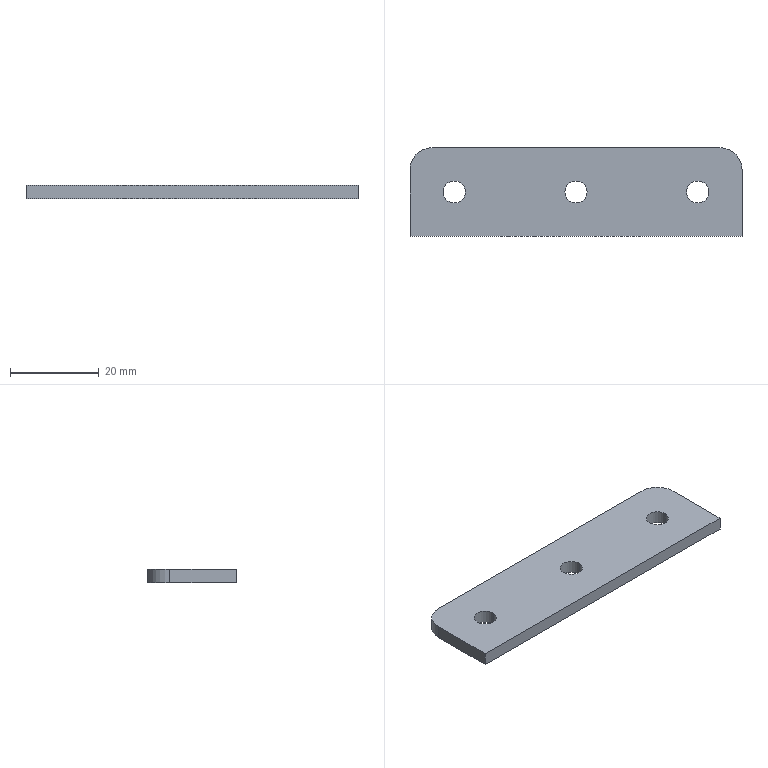Part | SolidWorks | features Extrusion 1, Fillet 1 | 1 solid | 14 faces | box 75 x 20 x 3 mm | volume 4291 mm3 | cylinder 8 | plane 6 | commonest cylinder face diameters 5 x6 10 x2
STEP:
#1=CARTESIAN_POINT('',(62.5,-10.,3.));
#2=VERTEX_POINT('',#1);
#3=CARTESIAN_POINT('',(67.5,-10.,3.));
#4=VERTEX_POINT('',#3);
#5=CARTESIAN_POINT('',(65.,-10.,3.));
#6=DIRECTION('',(0.,0.,1.));
#7=DIRECTION('',(1.,0.,0.));
#8=AXIS2_PLACEMENT_3D('',#5,#6,#7);
#9=CIRCLE('',#8,2.5);
#10=EDGE_CURVE('',#2,#4,#9,.T.);
#11=ORIENTED_EDGE('',*,*,#10,.T.);
#12=CARTESIAN_POINT('',(67.5,-10.,0.));
#13=VERTEX_POINT('',#12);
#14=CARTESIAN_POINT('',(67.5,-10.,3.));
#15=DIRECTION('',(0.,0.,-1.));
#16=VECTOR('',#15,1000.);
#17=LINE('',#14,#16);
#18=EDGE_CURVE('',#4,#13,#17,.T.);
#19=ORIENTED_EDGE('',*,*,#18,.T.);
#20=CARTESIAN_POINT('',(62.5,-10.,0.));
#21=VERTEX_POINT('',#20);
#22=CARTESIAN_POINT('',(65.,-10.,0.));
#23=DIRECTION('',(0.,0.,1.));
#24=DIRECTION('',(1.,0.,0.));
#25=AXIS2_PLACEMENT_3D('',#22,#23,#24);
#26=CIRCLE('',#25,2.5);
#27=EDGE_CURVE('',#21,#13,#26,.T.);
#28=ORIENTED_EDGE('',*,*,#27,.F.);
#29=CARTESIAN_POINT('',(62.5,-10.,3.));
#30=DIRECTION('',(0.,0.,-1.));
#31=VECTOR('',#30,1000.);
#32=LINE('',#29,#31);
#33=EDGE_CURVE('',#2,#21,#32,.T.);
#34=ORIENTED_EDGE('',*,*,#33,.F.);
#35=EDGE_LOOP('',(#11,#19,#28,#34));
#36=FACE_OUTER_BOUND('',#35,.T.);
#37=CARTESIAN_POINT('',(65.,-10.,3.));
#38=DIRECTION('',(0.,0.,-1.));
#39=DIRECTION('',(-1.,0.,0.));
#40=AXIS2_PLACEMENT_3D('',#37,#38,#39);
#41=CYLINDRICAL_SURFACE('',#40,2.5);
#42=ADVANCED_FACE('',(#36),#41,.F.);
#43=CARTESIAN_POINT('',(35.,-10.,3.));
#44=VERTEX_POINT('',#43);
#45=CARTESIAN_POINT('',(40.,-10.,3.));
#46=VERTEX_POINT('',#45);
#47=CARTESIAN_POINT('',(37.5,-10.,3.));
#48=DIRECTION('',(0.,0.,1.));
#49=DIRECTION('',(1.,0.,0.));
#50=AXIS2_PLACEMENT_3D('',#47,#48,#49);
#51=CIRCLE('',#50,2.5);
#52=EDGE_CURVE('',#44,#46,#51,.T.);
#53=ORIENTED_EDGE('',*,*,#52,.T.);
#54=CARTESIAN_POINT('',(40.,-10.,0.));
#55=VERTEX_POINT('',#54);
#56=CARTESIAN_POINT('',(40.,-10.,3.));
#57=DIRECTION('',(0.,0.,-1.));
#58=VECTOR('',#57,1000.);
#59=LINE('',#56,#58);
#60=EDGE_CURVE('',#46,#55,#59,.T.);
#61=ORIENTED_EDGE('',*,*,#60,.T.);
#62=CARTESIAN_POINT('',(35.,-10.,0.));
#63=VERTEX_POINT('',#62);
#64=CARTESIAN_POINT('',(37.5,-10.,0.));
#65=DIRECTION('',(0.,0.,1.));
#66=DIRECTION('',(1.,0.,0.));
#67=AXIS2_PLACEMENT_3D('',#64,#65,#66);
#68=CIRCLE('',#67,2.5);
#69=EDGE_CURVE('',#63,#55,#68,.T.);
#70=ORIENTED_EDGE('',*,*,#69,.F.);
#71=CARTESIAN_POINT('',(35.,-10.,3.));
#72=DIRECTION('',(0.,0.,-1.));
#73=VECTOR('',#72,1000.);
#74=LINE('',#71,#73);
#75=EDGE_CURVE('',#44,#63,#74,.T.);
#76=ORIENTED_EDGE('',*,*,#75,.F.);
#77=EDGE_LOOP('',(#53,#61,#70,#76));
#78=FACE_OUTER_BOUND('',#77,.T.);
#79=CARTESIAN_POINT('',(37.5,-10.,3.));
#80=DIRECTION('',(0.,0.,-1.));
#81=DIRECTION('',(-1.,0.,0.));
#82=AXIS2_PLACEMENT_3D('',#79,#80,#81);
#83=CYLINDRICAL_SURFACE('',#82,2.5);
#84=ADVANCED_FACE('',(#78),#83,.F.);
#85=CARTESIAN_POINT('',(7.5,-10.,3.));
#86=VERTEX_POINT('',#85);
#87=CARTESIAN_POINT('',(12.5,-10.,3.));
#88=VERTEX_POINT('',#87);
#89=CARTESIAN_POINT('',(10.,-10.,3.));
#90=DIRECTION('',(0.,0.,1.));
#91=DIRECTION('',(1.,0.,0.));
#92=AXIS2_PLACEMENT_3D('',#89,#90,#91);
#93=CIRCLE('',#92,2.5);
#94=EDGE_CURVE('',#86,#88,#93,.T.);
#95=ORIENTED_EDGE('',*,*,#94,.T.);
#96=CARTESIAN_POINT('',(12.5,-10.,0.));
#97=VERTEX_POINT('',#96);
#98=CARTESIAN_POINT('',(12.5,-10.,3.));
#99=DIRECTION('',(0.,0.,-1.));
#100=VECTOR('',#99,1000.);
#101=LINE('',#98,#100);
#102=EDGE_CURVE('',#88,#97,#101,.T.);
#103=ORIENTED_EDGE('',*,*,#102,.T.);
#104=CARTESIAN_POINT('',(7.5,-10.,0.));
#105=VERTEX_POINT('',#104);
#106=CARTESIAN_POINT('',(10.,-10.,0.));
#107=DIRECTION('',(0.,0.,1.));
#108=DIRECTION('',(1.,0.,0.));
#109=AXIS2_PLACEMENT_3D('',#106,#107,#108);
#110=CIRCLE('',#109,2.5);
#111=EDGE_CURVE('',#105,#97,#110,.T.);
#112=ORIENTED_EDGE('',*,*,#111,.F.);
#113=CARTESIAN_POINT('',(7.5,-10.,3.));
#114=DIRECTION('',(0.,0.,-1.));
#115=VECTOR('',#114,1000.);
#116=LINE('',#113,#115);
#117=EDGE_CURVE('',#86,#105,#116,.T.);
#118=ORIENTED_EDGE('',*,*,#117,.F.);
#119=EDGE_LOOP('',(#95,#103,#112,#118));
#120=FACE_OUTER_BOUND('',#119,.T.);
#121=CARTESIAN_POINT('',(10.,-10.,3.));
#122=DIRECTION('',(0.,0.,-1.));
#123=DIRECTION('',(-1.,0.,0.));
#124=AXIS2_PLACEMENT_3D('',#121,#122,#123);
#125=CYLINDRICAL_SURFACE('',#124,2.5);
#126=ADVANCED_FACE('',(#120),#125,.F.);
#127=ORIENTED_EDGE('',*,*,#52,.F.);
#128=CARTESIAN_POINT('',(37.5,-10.,3.));
#129=DIRECTION('',(0.,0.,1.));
#130=DIRECTION('',(1.,0.,0.));
#131=AXIS2_PLACEMENT_3D('',#128,#129,#130);
#132=CIRCLE('',#131,2.5);
#133=EDGE_CURVE('',#46,#44,#132,.T.);
#134=ORIENTED_EDGE('',*,*,#133,.F.);
#135=EDGE_LOOP('',(#127,#134));
#136=FACE_BOUND('',#135,.T.);
#137=CARTESIAN_POINT('',(75.,-20.,3.));
#138=VERTEX_POINT('',#137);
#139=CARTESIAN_POINT('',(75.,-5.,3.));
#140=VERTEX_POINT('',#139);
#141=CARTESIAN_POINT('',(75.,0.,3.));
#142=DIRECTION('',(0.,1.,0.));
#143=VECTOR('',#142,1000.);
#144=LINE('',#141,#143);
#145=EDGE_CURVE('',#138,#140,#144,.T.);
#146=ORIENTED_EDGE('',*,*,#145,.T.);
#147=CARTESIAN_POINT('',(70.,0.,3.));
#148=VERTEX_POINT('',#147);
#149=CARTESIAN_POINT('',(70.,-5.,3.));
#150=DIRECTION('',(0.,0.,1.));
#151=DIRECTION('',(1.,0.,0.));
#152=AXIS2_PLACEMENT_3D('',#149,#150,#151);
#153=CIRCLE('',#152,5.);
#154=EDGE_CURVE('',#140,#148,#153,.T.);
#155=ORIENTED_EDGE('',*,*,#154,.T.);
#156=CARTESIAN_POINT('',(5.,0.,3.));
#157=VERTEX_POINT('',#156);
#158=CARTESIAN_POINT('',(0.,0.,3.));
#159=DIRECTION('',(-1.,0.,0.));
#160=VECTOR('',#159,1000.);
#161=LINE('',#158,#160);
#162=EDGE_CURVE('',#148,#157,#161,.T.);
#163=ORIENTED_EDGE('',*,*,#162,.T.);
#164=CARTESIAN_POINT('',(0.,-5.,3.));
#165=VERTEX_POINT('',#164);
#166=CARTESIAN_POINT('',(5.,-5.,3.));
#167=DIRECTION('',(0.,0.,1.));
#168=DIRECTION('',(1.,0.,0.));
#169=AXIS2_PLACEMENT_3D('',#166,#167,#168);
#170=CIRCLE('',#169,5.);
#171=EDGE_CURVE('',#157,#165,#170,.T.);
#172=ORIENTED_EDGE('',*,*,#171,.T.);
#173=CARTESIAN_POINT('',(0.,-20.,3.));
#174=VERTEX_POINT('',#173);
#175=CARTESIAN_POINT('',(0.,0.,3.));
#176=DIRECTION('',(0.,-1.,0.));
#177=VECTOR('',#176,1000.);
#178=LINE('',#175,#177);
#179=EDGE_CURVE('',#165,#174,#178,.T.);
#180=ORIENTED_EDGE('',*,*,#179,.T.);
#181=CARTESIAN_POINT('',(0.,-20.,3.));
#182=DIRECTION('',(1.,0.,0.));
#183=VECTOR('',#182,1000.);
#184=LINE('',#181,#183);
#185=EDGE_CURVE('',#174,#138,#184,.T.);
#186=ORIENTED_EDGE('',*,*,#185,.T.);
#187=EDGE_LOOP('',(#146,#155,#163,#172,#180,#186));
#188=FACE_OUTER_BOUND('',#187,.T.);
#189=ORIENTED_EDGE('',*,*,#94,.F.);
#190=CARTESIAN_POINT('',(10.,-10.,3.));
#191=DIRECTION('',(0.,0.,1.));
#192=DIRECTION('',(1.,0.,0.));
#193=AXIS2_PLACEMENT_3D('',#190,#191,#192);
#194=CIRCLE('',#193,2.5);
#195=EDGE_CURVE('',#88,#86,#194,.T.);
#196=ORIENTED_EDGE('',*,*,#195,.F.);
#197=EDGE_LOOP('',(#189,#196));
#198=FACE_BOUND('',#197,.T.);
#199=ORIENTED_EDGE('',*,*,#10,.F.);
#200=CARTESIAN_POINT('',(65.,-10.,3.));
#201=DIRECTION('',(0.,0.,1.));
#202=DIRECTION('',(1.,0.,0.));
#203=AXIS2_PLACEMENT_3D('',#200,#201,#202);
#204=CIRCLE('',#203,2.5);
#205=EDGE_CURVE('',#4,#2,#204,.T.);
#206=ORIENTED_EDGE('',*,*,#205,.F.);
#207=EDGE_LOOP('',(#199,#206));
#208=FACE_BOUND('',#207,.T.);
#209=CARTESIAN_POINT('',(0.,0.,3.));
#210=DIRECTION('',(0.,0.,1.));
#211=DIRECTION('',(1.,0.,0.));
#212=AXIS2_PLACEMENT_3D('',#209,#210,#211);
#213=PLANE('',#212);
#214=ADVANCED_FACE('',(#136,#188,#198,#208),#213,.T.);
#215=CARTESIAN_POINT('',(70.,0.,0.));
#216=VERTEX_POINT('',#215);
#217=CARTESIAN_POINT('',(5.,0.,0.));
#218=VERTEX_POINT('',#217);
#219=CARTESIAN_POINT('',(0.,0.,0.));
#220=DIRECTION('',(-1.,0.,0.));
#221=VECTOR('',#220,1000.);
#222=LINE('',#219,#221);
#223=EDGE_CURVE('',#216,#218,#222,.T.);
#224=ORIENTED_EDGE('',*,*,#223,.F.);
#225=CARTESIAN_POINT('',(75.,-5.,0.));
#226=VERTEX_POINT('',#225);
#227=CARTESIAN_POINT('',(70.,-5.,0.));
#228=DIRECTION('',(0.,0.,-1.));
#229=DIRECTION('',(1.,0.,0.));
#230=AXIS2_PLACEMENT_3D('',#227,#228,#229);
#231=CIRCLE('',#230,5.);
#232=EDGE_CURVE('',#216,#226,#231,.T.);
#233=ORIENTED_EDGE('',*,*,#232,.T.);
#234=CARTESIAN_POINT('',(75.,-20.,0.));
#235=VERTEX_POINT('',#234);
#236=CARTESIAN_POINT('',(75.,0.,0.));
#237=DIRECTION('',(0.,1.,0.));
#238=VECTOR('',#237,1000.);
#239=LINE('',#236,#238);
#240=EDGE_CURVE('',#235,#226,#239,.T.);
#241=ORIENTED_EDGE('',*,*,#240,.F.);
#242=CARTESIAN_POINT('',(0.,-20.,0.));
#243=VERTEX_POINT('',#242);
#244=CARTESIAN_POINT('',(0.,-20.,0.));
#245=DIRECTION('',(1.,0.,0.));
#246=VECTOR('',#245,1000.);
#247=LINE('',#244,#246);
#248=EDGE_CURVE('',#243,#235,#247,.T.);
#249=ORIENTED_EDGE('',*,*,#248,.F.);
#250=CARTESIAN_POINT('',(0.,-5.,0.));
#251=VERTEX_POINT('',#250);
#252=CARTESIAN_POINT('',(0.,0.,0.));
#253=DIRECTION('',(0.,-1.,0.));
#254=VECTOR('',#253,1000.);
#255=LINE('',#252,#254);
#256=EDGE_CURVE('',#251,#243,#255,.T.);
#257=ORIENTED_EDGE('',*,*,#256,.F.);
#258=CARTESIAN_POINT('',(5.,-5.,0.));
#259=DIRECTION('',(0.,0.,-1.));
#260=DIRECTION('',(1.,0.,0.));
#261=AXIS2_PLACEMENT_3D('',#258,#259,#260);
#262=CIRCLE('',#261,5.);
#263=EDGE_CURVE('',#251,#218,#262,.T.);
#264=ORIENTED_EDGE('',*,*,#263,.T.);
#265=EDGE_LOOP('',(#224,#233,#241,#249,#257,#264));
#266=FACE_OUTER_BOUND('',#265,.T.);
#267=ORIENTED_EDGE('',*,*,#111,.T.);
#268=CARTESIAN_POINT('',(10.,-10.,0.));
#269=DIRECTION('',(0.,0.,1.));
#270=DIRECTION('',(1.,0.,0.));
#271=AXIS2_PLACEMENT_3D('',#268,#269,#270);
#272=CIRCLE('',#271,2.5);
#273=EDGE_CURVE('',#97,#105,#272,.T.);
#274=ORIENTED_EDGE('',*,*,#273,.T.);
#275=EDGE_LOOP('',(#267,#274));
#276=FACE_BOUND('',#275,.T.);
#277=ORIENTED_EDGE('',*,*,#69,.T.);
#278=CARTESIAN_POINT('',(37.5,-10.,0.));
#279=DIRECTION('',(0.,0.,1.));
#280=DIRECTION('',(1.,0.,0.));
#281=AXIS2_PLACEMENT_3D('',#278,#279,#280);
#282=CIRCLE('',#281,2.5);
#283=EDGE_CURVE('',#55,#63,#282,.T.);
#284=ORIENTED_EDGE('',*,*,#283,.T.);
#285=EDGE_LOOP('',(#277,#284));
#286=FACE_BOUND('',#285,.T.);
#287=ORIENTED_EDGE('',*,*,#27,.T.);
#288=CARTESIAN_POINT('',(65.,-10.,0.));
#289=DIRECTION('',(0.,0.,1.));
#290=DIRECTION('',(1.,0.,0.));
#291=AXIS2_PLACEMENT_3D('',#288,#289,#290);
#292=CIRCLE('',#291,2.5);
#293=EDGE_CURVE('',#13,#21,#292,.T.);
#294=ORIENTED_EDGE('',*,*,#293,.T.);
#295=EDGE_LOOP('',(#287,#294));
#296=FACE_BOUND('',#295,.T.);
#297=CARTESIAN_POINT('',(0.,0.,0.));
#298=DIRECTION('',(0.,0.,1.));
#299=DIRECTION('',(1.,0.,0.));
#300=AXIS2_PLACEMENT_3D('',#297,#298,#299);
#301=PLANE('',#300);
#302=ADVANCED_FACE('',(#266,#276,#286,#296),#301,.F.);
#303=ORIENTED_EDGE('',*,*,#179,.F.);
#304=CARTESIAN_POINT('',(0.,-5.,3.));
#305=DIRECTION('',(0.,0.,-1.));
#306=VECTOR('',#305,1000.);
#307=LINE('',#304,#306);
#308=EDGE_CURVE('',#165,#251,#307,.T.);
#309=ORIENTED_EDGE('',*,*,#308,.T.);
#310=ORIENTED_EDGE('',*,*,#256,.T.);
#311=CARTESIAN_POINT('',(0.,-20.,3.));
#312=DIRECTION('',(0.,0.,-1.));
#313=VECTOR('',#312,1000.);
#314=LINE('',#311,#313);
#315=EDGE_CURVE('',#174,#243,#314,.T.);
#316=ORIENTED_EDGE('',*,*,#315,.F.);
#317=EDGE_LOOP('',(#303,#309,#310,#316));
#318=FACE_OUTER_BOUND('',#317,.T.);
#319=CARTESIAN_POINT('',(0.,0.,3.));
#320=DIRECTION('',(1.,0.,0.));
#321=DIRECTION('',(0.,1.,0.));
#322=AXIS2_PLACEMENT_3D('',#319,#320,#321);
#323=PLANE('',#322);
#324=ADVANCED_FACE('',(#318),#323,.F.);
#325=ORIENTED_EDGE('',*,*,#248,.T.);
#326=CARTESIAN_POINT('',(75.,-20.,3.));
#327=DIRECTION('',(0.,0.,-1.));
#328=VECTOR('',#327,1000.);
#329=LINE('',#326,#328);
#330=EDGE_CURVE('',#138,#235,#329,.T.);
#331=ORIENTED_EDGE('',*,*,#330,.F.);
#332=ORIENTED_EDGE('',*,*,#185,.F.);
#333=ORIENTED_EDGE('',*,*,#315,.T.);
#334=EDGE_LOOP('',(#325,#331,#332,#333));
#335=FACE_OUTER_BOUND('',#334,.T.);
#336=CARTESIAN_POINT('',(0.,-20.,3.));
#337=DIRECTION('',(0.,1.,0.));
#338=DIRECTION('',(0.,0.,1.));
#339=AXIS2_PLACEMENT_3D('',#336,#337,#338);
#340=PLANE('',#339);
#341=ADVANCED_FACE('',(#335),#340,.F.);
#342=ORIENTED_EDGE('',*,*,#240,.T.);
#343=CARTESIAN_POINT('',(75.,-5.,3.));
#344=DIRECTION('',(0.,0.,1.));
#345=VECTOR('',#344,1000.);
#346=LINE('',#343,#345);
#347=EDGE_CURVE('',#226,#140,#346,.T.);
#348=ORIENTED_EDGE('',*,*,#347,.T.);
#349=ORIENTED_EDGE('',*,*,#145,.F.);
#350=ORIENTED_EDGE('',*,*,#330,.T.);
#351=EDGE_LOOP('',(#342,#348,#349,#350));
#352=FACE_OUTER_BOUND('',#351,.T.);
#353=CARTESIAN_POINT('',(75.,0.,3.));
#354=DIRECTION('',(-1.,0.,0.));
#355=DIRECTION('',(0.,0.,1.));
#356=AXIS2_PLACEMENT_3D('',#353,#354,#355);
#357=PLANE('',#356);
#358=ADVANCED_FACE('',(#352),#357,.F.);
#359=ORIENTED_EDGE('',*,*,#162,.F.);
#360=CARTESIAN_POINT('',(70.,0.,3.));
#361=DIRECTION('',(0.,0.,-1.));
#362=VECTOR('',#361,1000.);
#363=LINE('',#360,#362);
#364=EDGE_CURVE('',#148,#216,#363,.T.);
#365=ORIENTED_EDGE('',*,*,#364,.T.);
#366=ORIENTED_EDGE('',*,*,#223,.T.);
#367=CARTESIAN_POINT('',(5.,0.,3.));
#368=DIRECTION('',(0.,0.,1.));
#369=VECTOR('',#368,1000.);
#370=LINE('',#367,#369);
#371=EDGE_CURVE('',#218,#157,#370,.T.);
#372=ORIENTED_EDGE('',*,*,#371,.T.);
#373=EDGE_LOOP('',(#359,#365,#366,#372));
#374=FACE_OUTER_BOUND('',#373,.T.);
#375=CARTESIAN_POINT('',(0.,0.,3.));
#376=DIRECTION('',(0.,-1.,0.));
#377=DIRECTION('',(0.,0.,-1.));
#378=AXIS2_PLACEMENT_3D('',#375,#376,#377);
#379=PLANE('',#378);
#380=ADVANCED_FACE('',(#374),#379,.F.);
#381=ORIENTED_EDGE('',*,*,#102,.F.);
#382=ORIENTED_EDGE('',*,*,#195,.T.);
#383=ORIENTED_EDGE('',*,*,#117,.T.);
#384=ORIENTED_EDGE('',*,*,#273,.F.);
#385=EDGE_LOOP('',(#381,#382,#383,#384));
#386=FACE_OUTER_BOUND('',#385,.T.);
#387=CARTESIAN_POINT('',(10.,-10.,3.));
#388=DIRECTION('',(0.,0.,-1.));
#389=DIRECTION('',(-1.,0.,0.));
#390=AXIS2_PLACEMENT_3D('',#387,#388,#389);
#391=CYLINDRICAL_SURFACE('',#390,2.5);
#392=ADVANCED_FACE('',(#386),#391,.F.);
#393=ORIENTED_EDGE('',*,*,#60,.F.);
#394=ORIENTED_EDGE('',*,*,#133,.T.);
#395=ORIENTED_EDGE('',*,*,#75,.T.);
#396=ORIENTED_EDGE('',*,*,#283,.F.);
#397=EDGE_LOOP('',(#393,#394,#395,#396));
#398=FACE_OUTER_BOUND('',#397,.T.);
#399=CARTESIAN_POINT('',(37.5,-10.,3.));
#400=DIRECTION('',(0.,0.,-1.));
#401=DIRECTION('',(-1.,0.,0.));
#402=AXIS2_PLACEMENT_3D('',#399,#400,#401);
#403=CYLINDRICAL_SURFACE('',#402,2.5);
#404=ADVANCED_FACE('',(#398),#403,.F.);
#405=ORIENTED_EDGE('',*,*,#18,.F.);
#406=ORIENTED_EDGE('',*,*,#205,.T.);
#407=ORIENTED_EDGE('',*,*,#33,.T.);
#408=ORIENTED_EDGE('',*,*,#293,.F.);
#409=EDGE_LOOP('',(#405,#406,#407,#408));
#410=FACE_OUTER_BOUND('',#409,.T.);
#411=CARTESIAN_POINT('',(65.,-10.,3.));
#412=DIRECTION('',(0.,0.,-1.));
#413=DIRECTION('',(-1.,0.,0.));
#414=AXIS2_PLACEMENT_3D('',#411,#412,#413);
#415=CYLINDRICAL_SURFACE('',#414,2.5);
#416=ADVANCED_FACE('',(#410),#415,.F.);
#417=ORIENTED_EDGE('',*,*,#154,.F.);
#418=ORIENTED_EDGE('',*,*,#347,.F.);
#419=ORIENTED_EDGE('',*,*,#232,.F.);
#420=ORIENTED_EDGE('',*,*,#364,.F.);
#421=EDGE_LOOP('',(#417,#418,#419,#420));
#422=FACE_OUTER_BOUND('',#421,.T.);
#423=CARTESIAN_POINT('',(70.,-5.,3.));
#424=DIRECTION('',(0.,0.,-1.));
#425=DIRECTION('',(-1.,0.,0.));
#426=AXIS2_PLACEMENT_3D('',#423,#424,#425);
#427=CYLINDRICAL_SURFACE('',#426,5.);
#428=ADVANCED_FACE('',(#422),#427,.T.);
#429=ORIENTED_EDGE('',*,*,#171,.F.);
#430=ORIENTED_EDGE('',*,*,#371,.F.);
#431=ORIENTED_EDGE('',*,*,#263,.F.);
#432=ORIENTED_EDGE('',*,*,#308,.F.);
#433=EDGE_LOOP('',(#429,#430,#431,#432));
#434=FACE_OUTER_BOUND('',#433,.T.);
#435=CARTESIAN_POINT('',(5.,-5.,3.));
#436=DIRECTION('',(0.,0.,-1.));
#437=DIRECTION('',(-1.,0.,0.));
#438=AXIS2_PLACEMENT_3D('',#435,#436,#437);
#439=CYLINDRICAL_SURFACE('',#438,5.);
#440=ADVANCED_FACE('',(#434),#439,.T.);
#441=CLOSED_SHELL('',(#42,#84,#126,#214,#302,#324,#341,#358,#380,#392,#404,#416,#428,#440));
#442=MANIFOLD_SOLID_BREP('',#441);
#443=CARTESIAN_POINT('',(0.,0.,0.));
#444=DIRECTION('',(0.,0.,1.));
#445=DIRECTION('',(1.,0.,0.));
#446=AXIS2_PLACEMENT_3D('',#443,#444,#445);
#447=(LENGTH_UNIT()NAMED_UNIT(*)SI_UNIT(.MILLI.,.METRE.));
#448=UNCERTAINTY_MEASURE_WITH_UNIT(LENGTH_MEASURE(0.00001),#447,'','');
#449=(NAMED_UNIT(*)PLANE_ANGLE_UNIT()SI_UNIT($,.RADIAN.));
#450=(NAMED_UNIT(*)SI_UNIT($,.STERADIAN.)SOLID_ANGLE_UNIT());
#451=(GEOMETRIC_REPRESENTATION_CONTEXT(3)GLOBAL_UNCERTAINTY_ASSIGNED_CONTEXT((#448))GLOBAL_UNIT_ASSIGNED_CONTEXT((#447,#449,#450))REPRESENTATION_CONTEXT('',''));
#452=ADVANCED_BREP_SHAPE_REPRESENTATION('',(#442,#446),#451);